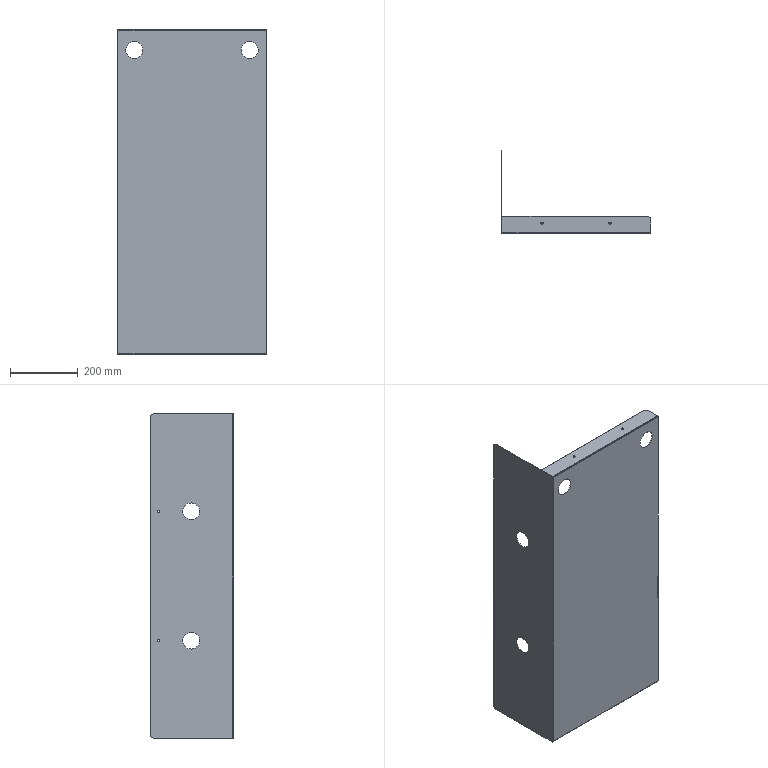Part | SolidWorks | features BaseBody 1 | 1 solid | 48 faces | box 440 x 245 x 955 mm | volume 1029152 mm3 | cylinder 30 | plane 18 | commonest cylinder face diameters 6.6 x12 50 x8 20 x4 1 x3 4 x3
STEP:
#1=CARTESIAN_POINT('',(50.,0.,870.));
#2=VERTEX_POINT('',#1);
#3=CARTESIAN_POINT('',(50.,0.,920.));
#4=VERTEX_POINT('',#3);
#5=CARTESIAN_POINT('',(50.,0.,895.));
#6=DIRECTION('',(0.,1.,0.));
#7=DIRECTION('',(0.,0.,1.));
#8=AXIS2_PLACEMENT_3D('',#5,#6,#7);
#9=CIRCLE('',#8,25.);
#10=EDGE_CURVE('',#2,#4,#9,.T.);
#11=ORIENTED_EDGE('',*,*,#10,.F.);
#12=CARTESIAN_POINT('',(50.,1.5,870.));
#13=VERTEX_POINT('',#12);
#14=CARTESIAN_POINT('',(50.,1.5,870.));
#15=DIRECTION('',(0.,1.,0.));
#16=VECTOR('',#15,1000.);
#17=LINE('',#14,#16);
#18=EDGE_CURVE('',#2,#13,#17,.T.);
#19=ORIENTED_EDGE('',*,*,#18,.T.);
#20=CARTESIAN_POINT('',(50.,1.5,920.));
#21=VERTEX_POINT('',#20);
#22=CARTESIAN_POINT('',(50.,1.5,895.));
#23=DIRECTION('',(0.,-1.,0.));
#24=DIRECTION('',(0.,0.,1.));
#25=AXIS2_PLACEMENT_3D('',#22,#23,#24);
#26=CIRCLE('',#25,25.);
#27=EDGE_CURVE('',#21,#13,#26,.T.);
#28=ORIENTED_EDGE('',*,*,#27,.F.);
#29=CARTESIAN_POINT('',(50.,1.5,920.));
#30=DIRECTION('',(0.,1.,0.));
#31=VECTOR('',#30,1000.);
#32=LINE('',#29,#31);
#33=EDGE_CURVE('',#4,#21,#32,.T.);
#34=ORIENTED_EDGE('',*,*,#33,.F.);
#35=EDGE_LOOP('',(#11,#19,#28,#34));
#36=FACE_OUTER_BOUND('',#35,.T.);
#37=CARTESIAN_POINT('',(50.,1.5,895.));
#38=DIRECTION('',(0.,1.,0.));
#39=DIRECTION('',(0.,0.,1.));
#40=AXIS2_PLACEMENT_3D('',#37,#38,#39);
#41=CYLINDRICAL_SURFACE('',#40,25.);
#42=ADVANCED_FACE('',(#36),#41,.F.);
#43=CARTESIAN_POINT('',(390.,0.,870.));
#44=VERTEX_POINT('',#43);
#45=CARTESIAN_POINT('',(390.,0.,920.));
#46=VERTEX_POINT('',#45);
#47=CARTESIAN_POINT('',(390.,0.,895.));
#48=DIRECTION('',(0.,1.,0.));
#49=DIRECTION('',(0.,0.,1.));
#50=AXIS2_PLACEMENT_3D('',#47,#48,#49);
#51=CIRCLE('',#50,25.);
#52=EDGE_CURVE('',#44,#46,#51,.T.);
#53=ORIENTED_EDGE('',*,*,#52,.F.);
#54=CARTESIAN_POINT('',(390.,1.5,870.));
#55=VERTEX_POINT('',#54);
#56=CARTESIAN_POINT('',(390.,1.5,870.));
#57=DIRECTION('',(0.,1.,0.));
#58=VECTOR('',#57,1000.);
#59=LINE('',#56,#58);
#60=EDGE_CURVE('',#44,#55,#59,.T.);
#61=ORIENTED_EDGE('',*,*,#60,.T.);
#62=CARTESIAN_POINT('',(390.,1.5,920.));
#63=VERTEX_POINT('',#62);
#64=CARTESIAN_POINT('',(390.,1.5,895.));
#65=DIRECTION('',(0.,-1.,0.));
#66=DIRECTION('',(0.,0.,1.));
#67=AXIS2_PLACEMENT_3D('',#64,#65,#66);
#68=CIRCLE('',#67,25.);
#69=EDGE_CURVE('',#63,#55,#68,.T.);
#70=ORIENTED_EDGE('',*,*,#69,.F.);
#71=CARTESIAN_POINT('',(390.,1.5,920.));
#72=DIRECTION('',(0.,1.,0.));
#73=VECTOR('',#72,1000.);
#74=LINE('',#71,#73);
#75=EDGE_CURVE('',#46,#63,#74,.T.);
#76=ORIENTED_EDGE('',*,*,#75,.F.);
#77=EDGE_LOOP('',(#53,#61,#70,#76));
#78=FACE_OUTER_BOUND('',#77,.T.);
#79=CARTESIAN_POINT('',(390.,1.5,895.));
#80=DIRECTION('',(0.,1.,0.));
#81=DIRECTION('',(0.,0.,1.));
#82=AXIS2_PLACEMENT_3D('',#79,#80,#81);
#83=CYLINDRICAL_SURFACE('',#82,25.);
#84=ADVANCED_FACE('',(#78),#83,.F.);
#85=CARTESIAN_POINT('',(316.7,30.,953.5));
#86=VERTEX_POINT('',#85);
#87=CARTESIAN_POINT('',(323.3,30.,953.5));
#88=VERTEX_POINT('',#87);
#89=CARTESIAN_POINT('',(320.,30.,953.5));
#90=DIRECTION('',(0.,0.,1.));
#91=DIRECTION('',(1.,0.,0.));
#92=AXIS2_PLACEMENT_3D('',#89,#90,#91);
#93=CIRCLE('',#92,3.3);
#94=EDGE_CURVE('',#86,#88,#93,.T.);
#95=ORIENTED_EDGE('',*,*,#94,.F.);
#96=CARTESIAN_POINT('',(316.7,30.,955.));
#97=VERTEX_POINT('',#96);
#98=CARTESIAN_POINT('',(316.7,30.,955.));
#99=DIRECTION('',(0.,0.,1.));
#100=VECTOR('',#99,1000.);
#101=LINE('',#98,#100);
#102=EDGE_CURVE('',#86,#97,#101,.T.);
#103=ORIENTED_EDGE('',*,*,#102,.T.);
#104=CARTESIAN_POINT('',(323.3,30.,955.));
#105=VERTEX_POINT('',#104);
#106=CARTESIAN_POINT('',(320.,30.,955.));
#107=DIRECTION('',(0.,0.,-1.));
#108=DIRECTION('',(1.,0.,0.));
#109=AXIS2_PLACEMENT_3D('',#106,#107,#108);
#110=CIRCLE('',#109,3.3);
#111=EDGE_CURVE('',#105,#97,#110,.T.);
#112=ORIENTED_EDGE('',*,*,#111,.F.);
#113=CARTESIAN_POINT('',(323.3,30.,955.));
#114=DIRECTION('',(0.,0.,1.));
#115=VECTOR('',#114,1000.);
#116=LINE('',#113,#115);
#117=EDGE_CURVE('',#88,#105,#116,.T.);
#118=ORIENTED_EDGE('',*,*,#117,.F.);
#119=EDGE_LOOP('',(#95,#103,#112,#118));
#120=FACE_OUTER_BOUND('',#119,.T.);
#121=CARTESIAN_POINT('',(320.,30.,955.));
#122=DIRECTION('',(0.,0.,1.));
#123=DIRECTION('',(1.,0.,0.));
#124=AXIS2_PLACEMENT_3D('',#121,#122,#123);
#125=CYLINDRICAL_SURFACE('',#124,3.3);
#126=ADVANCED_FACE('',(#120),#125,.F.);
#127=CARTESIAN_POINT('',(116.7,30.,953.5));
#128=VERTEX_POINT('',#127);
#129=CARTESIAN_POINT('',(123.3,30.,953.5));
#130=VERTEX_POINT('',#129);
#131=CARTESIAN_POINT('',(120.,30.,953.5));
#132=DIRECTION('',(0.,0.,1.));
#133=DIRECTION('',(1.,0.,0.));
#134=AXIS2_PLACEMENT_3D('',#131,#132,#133);
#135=CIRCLE('',#134,3.3);
#136=EDGE_CURVE('',#128,#130,#135,.T.);
#137=ORIENTED_EDGE('',*,*,#136,.F.);
#138=CARTESIAN_POINT('',(116.7,30.,955.));
#139=VERTEX_POINT('',#138);
#140=CARTESIAN_POINT('',(116.7,30.,955.));
#141=DIRECTION('',(0.,0.,1.));
#142=VECTOR('',#141,1000.);
#143=LINE('',#140,#142);
#144=EDGE_CURVE('',#128,#139,#143,.T.);
#145=ORIENTED_EDGE('',*,*,#144,.T.);
#146=CARTESIAN_POINT('',(123.3,30.,955.));
#147=VERTEX_POINT('',#146);
#148=CARTESIAN_POINT('',(120.,30.,955.));
#149=DIRECTION('',(0.,0.,-1.));
#150=DIRECTION('',(1.,0.,0.));
#151=AXIS2_PLACEMENT_3D('',#148,#149,#150);
#152=CIRCLE('',#151,3.3);
#153=EDGE_CURVE('',#147,#139,#152,.T.);
#154=ORIENTED_EDGE('',*,*,#153,.F.);
#155=CARTESIAN_POINT('',(123.3,30.,955.));
#156=DIRECTION('',(0.,0.,1.));
#157=VECTOR('',#156,1000.);
#158=LINE('',#155,#157);
#159=EDGE_CURVE('',#130,#147,#158,.T.);
#160=ORIENTED_EDGE('',*,*,#159,.F.);
#161=EDGE_LOOP('',(#137,#145,#154,#160));
#162=FACE_OUTER_BOUND('',#161,.T.);
#163=CARTESIAN_POINT('',(120.,30.,955.));
#164=DIRECTION('',(0.,0.,1.));
#165=DIRECTION('',(1.,0.,0.));
#166=AXIS2_PLACEMENT_3D('',#163,#164,#165);
#167=CYLINDRICAL_SURFACE('',#166,3.3);
#168=ADVANCED_FACE('',(#162),#167,.F.);
#169=CARTESIAN_POINT('',(0.,125.,312.5));
#170=VERTEX_POINT('',#169);
#171=CARTESIAN_POINT('',(0.,125.,262.5));
#172=VERTEX_POINT('',#171);
#173=CARTESIAN_POINT('',(0.,125.,287.5));
#174=DIRECTION('',(1.,0.,0.));
#175=DIRECTION('',(0.,0.,-1.));
#176=AXIS2_PLACEMENT_3D('',#173,#174,#175);
#177=CIRCLE('',#176,25.);
#178=EDGE_CURVE('',#170,#172,#177,.T.);
#179=ORIENTED_EDGE('',*,*,#178,.F.);
#180=CARTESIAN_POINT('',(1.5,125.,312.5));
#181=VERTEX_POINT('',#180);
#182=CARTESIAN_POINT('',(1.5,125.,312.5));
#183=DIRECTION('',(1.,0.,0.));
#184=VECTOR('',#183,1000.);
#185=LINE('',#182,#184);
#186=EDGE_CURVE('',#170,#181,#185,.T.);
#187=ORIENTED_EDGE('',*,*,#186,.T.);
#188=CARTESIAN_POINT('',(1.5,125.,262.5));
#189=VERTEX_POINT('',#188);
#190=CARTESIAN_POINT('',(1.5,125.,287.5));
#191=DIRECTION('',(-1.,0.,0.));
#192=DIRECTION('',(0.,0.,-1.));
#193=AXIS2_PLACEMENT_3D('',#190,#191,#192);
#194=CIRCLE('',#193,25.);
#195=EDGE_CURVE('',#189,#181,#194,.T.);
#196=ORIENTED_EDGE('',*,*,#195,.F.);
#197=CARTESIAN_POINT('',(1.5,125.,262.5));
#198=DIRECTION('',(1.,0.,0.));
#199=VECTOR('',#198,1000.);
#200=LINE('',#197,#199);
#201=EDGE_CURVE('',#172,#189,#200,.T.);
#202=ORIENTED_EDGE('',*,*,#201,.F.);
#203=EDGE_LOOP('',(#179,#187,#196,#202));
#204=FACE_OUTER_BOUND('',#203,.T.);
#205=CARTESIAN_POINT('',(1.5,125.,287.5));
#206=DIRECTION('',(1.,0.,0.));
#207=DIRECTION('',(0.,0.,-1.));
#208=AXIS2_PLACEMENT_3D('',#205,#206,#207);
#209=CYLINDRICAL_SURFACE('',#208,25.);
#210=ADVANCED_FACE('',(#204),#209,.F.);
#211=CARTESIAN_POINT('',(0.,125.,692.5));
#212=VERTEX_POINT('',#211);
#213=CARTESIAN_POINT('',(0.,125.,642.5));
#214=VERTEX_POINT('',#213);
#215=CARTESIAN_POINT('',(0.,125.,667.5));
#216=DIRECTION('',(1.,0.,0.));
#217=DIRECTION('',(0.,0.,-1.));
#218=AXIS2_PLACEMENT_3D('',#215,#216,#217);
#219=CIRCLE('',#218,25.);
#220=EDGE_CURVE('',#212,#214,#219,.T.);
#221=ORIENTED_EDGE('',*,*,#220,.F.);
#222=CARTESIAN_POINT('',(1.5,125.,692.5));
#223=VERTEX_POINT('',#222);
#224=CARTESIAN_POINT('',(1.5,125.,692.5));
#225=DIRECTION('',(1.,0.,0.));
#226=VECTOR('',#225,1000.);
#227=LINE('',#224,#226);
#228=EDGE_CURVE('',#212,#223,#227,.T.);
#229=ORIENTED_EDGE('',*,*,#228,.T.);
#230=CARTESIAN_POINT('',(1.5,125.,642.5));
#231=VERTEX_POINT('',#230);
#232=CARTESIAN_POINT('',(1.5,125.,667.5));
#233=DIRECTION('',(-1.,0.,0.));
#234=DIRECTION('',(0.,0.,-1.));
#235=AXIS2_PLACEMENT_3D('',#232,#233,#234);
#236=CIRCLE('',#235,25.);
#237=EDGE_CURVE('',#231,#223,#236,.T.);
#238=ORIENTED_EDGE('',*,*,#237,.F.);
#239=CARTESIAN_POINT('',(1.5,125.,642.5));
#240=DIRECTION('',(1.,0.,0.));
#241=VECTOR('',#240,1000.);
#242=LINE('',#239,#241);
#243=EDGE_CURVE('',#214,#231,#242,.T.);
#244=ORIENTED_EDGE('',*,*,#243,.F.);
#245=EDGE_LOOP('',(#221,#229,#238,#244));
#246=FACE_OUTER_BOUND('',#245,.T.);
#247=CARTESIAN_POINT('',(1.5,125.,667.5));
#248=DIRECTION('',(1.,0.,0.));
#249=DIRECTION('',(0.,0.,-1.));
#250=AXIS2_PLACEMENT_3D('',#247,#248,#249);
#251=CYLINDRICAL_SURFACE('',#250,25.);
#252=ADVANCED_FACE('',(#246),#251,.F.);
#253=CARTESIAN_POINT('',(0.,220.,290.8));
#254=VERTEX_POINT('',#253);
#255=CARTESIAN_POINT('',(0.,220.,284.2));
#256=VERTEX_POINT('',#255);
#257=CARTESIAN_POINT('',(0.,220.,287.5));
#258=DIRECTION('',(1.,0.,0.));
#259=DIRECTION('',(0.,0.,-1.));
#260=AXIS2_PLACEMENT_3D('',#257,#258,#259);
#261=CIRCLE('',#260,3.3);
#262=EDGE_CURVE('',#254,#256,#261,.T.);
#263=ORIENTED_EDGE('',*,*,#262,.F.);
#264=CARTESIAN_POINT('',(1.5,220.,290.8));
#265=VERTEX_POINT('',#264);
#266=CARTESIAN_POINT('',(1.5,220.,290.8));
#267=DIRECTION('',(1.,0.,0.));
#268=VECTOR('',#267,1000.);
#269=LINE('',#266,#268);
#270=EDGE_CURVE('',#254,#265,#269,.T.);
#271=ORIENTED_EDGE('',*,*,#270,.T.);
#272=CARTESIAN_POINT('',(1.5,220.,284.2));
#273=VERTEX_POINT('',#272);
#274=CARTESIAN_POINT('',(1.5,220.,287.5));
#275=DIRECTION('',(-1.,0.,0.));
#276=DIRECTION('',(0.,0.,-1.));
#277=AXIS2_PLACEMENT_3D('',#274,#275,#276);
#278=CIRCLE('',#277,3.3);
#279=EDGE_CURVE('',#273,#265,#278,.T.);
#280=ORIENTED_EDGE('',*,*,#279,.F.);
#281=CARTESIAN_POINT('',(1.5,220.,284.2));
#282=DIRECTION('',(1.,0.,0.));
#283=VECTOR('',#282,1000.);
#284=LINE('',#281,#283);
#285=EDGE_CURVE('',#256,#273,#284,.T.);
#286=ORIENTED_EDGE('',*,*,#285,.F.);
#287=EDGE_LOOP('',(#263,#271,#280,#286));
#288=FACE_OUTER_BOUND('',#287,.T.);
#289=CARTESIAN_POINT('',(1.5,220.,287.5));
#290=DIRECTION('',(1.,0.,0.));
#291=DIRECTION('',(0.,0.,-1.));
#292=AXIS2_PLACEMENT_3D('',#289,#290,#291);
#293=CYLINDRICAL_SURFACE('',#292,3.3);
#294=ADVANCED_FACE('',(#288),#293,.F.);
#295=CARTESIAN_POINT('',(0.,220.,670.8));
#296=VERTEX_POINT('',#295);
#297=CARTESIAN_POINT('',(0.,220.,664.2));
#298=VERTEX_POINT('',#297);
#299=CARTESIAN_POINT('',(0.,220.,667.5));
#300=DIRECTION('',(1.,0.,0.));
#301=DIRECTION('',(0.,0.,-1.));
#302=AXIS2_PLACEMENT_3D('',#299,#300,#301);
#303=CIRCLE('',#302,3.3);
#304=EDGE_CURVE('',#296,#298,#303,.T.);
#305=ORIENTED_EDGE('',*,*,#304,.F.);
#306=CARTESIAN_POINT('',(1.5,220.,670.8));
#307=VERTEX_POINT('',#306);
#308=CARTESIAN_POINT('',(1.5,220.,670.8));
#309=DIRECTION('',(1.,0.,0.));
#310=VECTOR('',#309,1000.);
#311=LINE('',#308,#310);
#312=EDGE_CURVE('',#296,#307,#311,.T.);
#313=ORIENTED_EDGE('',*,*,#312,.T.);
#314=CARTESIAN_POINT('',(1.5,220.,664.2));
#315=VERTEX_POINT('',#314);
#316=CARTESIAN_POINT('',(1.5,220.,667.5));
#317=DIRECTION('',(-1.,0.,0.));
#318=DIRECTION('',(0.,0.,-1.));
#319=AXIS2_PLACEMENT_3D('',#316,#317,#318);
#320=CIRCLE('',#319,3.3);
#321=EDGE_CURVE('',#315,#307,#320,.T.);
#322=ORIENTED_EDGE('',*,*,#321,.F.);
#323=CARTESIAN_POINT('',(1.5,220.,664.2));
#324=DIRECTION('',(1.,0.,0.));
#325=VECTOR('',#324,1000.);
#326=LINE('',#323,#325);
#327=EDGE_CURVE('',#298,#315,#326,.T.);
#328=ORIENTED_EDGE('',*,*,#327,.F.);
#329=EDGE_LOOP('',(#305,#313,#322,#328));
#330=FACE_OUTER_BOUND('',#329,.T.);
#331=CARTESIAN_POINT('',(1.5,220.,667.5));
#332=DIRECTION('',(1.,0.,0.));
#333=DIRECTION('',(0.,0.,-1.));
#334=AXIS2_PLACEMENT_3D('',#331,#332,#333);
#335=CYLINDRICAL_SURFACE('',#334,3.3);
#336=ADVANCED_FACE('',(#330),#335,.F.);
#337=CARTESIAN_POINT('',(316.7,30.,0.));
#338=VERTEX_POINT('',#337);
#339=CARTESIAN_POINT('',(323.3,30.,0.));
#340=VERTEX_POINT('',#339);
#341=CARTESIAN_POINT('',(320.,30.,0.));
#342=DIRECTION('',(0.,0.,1.));
#343=DIRECTION('',(1.,0.,0.));
#344=AXIS2_PLACEMENT_3D('',#341,#342,#343);
#345=CIRCLE('',#344,3.3);
#346=EDGE_CURVE('',#338,#340,#345,.T.);
#347=ORIENTED_EDGE('',*,*,#346,.F.);
#348=CARTESIAN_POINT('',(316.7,30.,1.5));
#349=VERTEX_POINT('',#348);
#350=CARTESIAN_POINT('',(316.7,30.,955.));
#351=DIRECTION('',(0.,0.,1.));
#352=VECTOR('',#351,1000.);
#353=LINE('',#350,#352);
#354=EDGE_CURVE('',#338,#349,#353,.T.);
#355=ORIENTED_EDGE('',*,*,#354,.T.);
#356=CARTESIAN_POINT('',(323.3,30.,1.5));
#357=VERTEX_POINT('',#356);
#358=CARTESIAN_POINT('',(320.,30.,1.5));
#359=DIRECTION('',(0.,0.,-1.));
#360=DIRECTION('',(1.,0.,0.));
#361=AXIS2_PLACEMENT_3D('',#358,#359,#360);
#362=CIRCLE('',#361,3.3);
#363=EDGE_CURVE('',#357,#349,#362,.T.);
#364=ORIENTED_EDGE('',*,*,#363,.F.);
#365=CARTESIAN_POINT('',(323.3,30.,955.));
#366=DIRECTION('',(0.,0.,1.));
#367=VECTOR('',#366,1000.);
#368=LINE('',#365,#367);
#369=EDGE_CURVE('',#340,#357,#368,.T.);
#370=ORIENTED_EDGE('',*,*,#369,.F.);
#371=EDGE_LOOP('',(#347,#355,#364,#370));
#372=FACE_OUTER_BOUND('',#371,.T.);
#373=CARTESIAN_POINT('',(320.,30.,955.));
#374=DIRECTION('',(0.,0.,1.));
#375=DIRECTION('',(1.,0.,0.));
#376=AXIS2_PLACEMENT_3D('',#373,#374,#375);
#377=CYLINDRICAL_SURFACE('',#376,3.3);
#378=ADVANCED_FACE('',(#372),#377,.F.);
#379=CARTESIAN_POINT('',(116.7,30.,0.));
#380=VERTEX_POINT('',#379);
#381=CARTESIAN_POINT('',(123.3,30.,0.));
#382=VERTEX_POINT('',#381);
#383=CARTESIAN_POINT('',(120.,30.,0.));
#384=DIRECTION('',(0.,0.,1.));
#385=DIRECTION('',(1.,0.,0.));
#386=AXIS2_PLACEMENT_3D('',#383,#384,#385);
#387=CIRCLE('',#386,3.3);
#388=EDGE_CURVE('',#380,#382,#387,.T.);
#389=ORIENTED_EDGE('',*,*,#388,.F.);
#390=CARTESIAN_POINT('',(116.7,30.,1.5));
#391=VERTEX_POINT('',#390);
#392=CARTESIAN_POINT('',(116.7,30.,955.));
#393=DIRECTION('',(0.,0.,1.));
#394=VECTOR('',#393,1000.);
#395=LINE('',#392,#394);
#396=EDGE_CURVE('',#380,#391,#395,.T.);
#397=ORIENTED_EDGE('',*,*,#396,.T.);
#398=CARTESIAN_POINT('',(123.3,30.,1.5));
#399=VERTEX_POINT('',#398);
#400=CARTESIAN_POINT('',(120.,30.,1.5));
#401=DIRECTION('',(0.,0.,-1.));
#402=DIRECTION('',(1.,0.,0.));
#403=AXIS2_PLACEMENT_3D('',#400,#401,#402);
#404=CIRCLE('',#403,3.3);
#405=EDGE_CURVE('',#399,#391,#404,.T.);
#406=ORIENTED_EDGE('',*,*,#405,.F.);
#407=CARTESIAN_POINT('',(123.3,30.,955.));
#408=DIRECTION('',(0.,0.,1.));
#409=VECTOR('',#408,1000.);
#410=LINE('',#407,#409);
#411=EDGE_CURVE('',#382,#399,#410,.T.);
#412=ORIENTED_EDGE('',*,*,#411,.F.);
#413=EDGE_LOOP('',(#389,#397,#406,#412));
#414=FACE_OUTER_BOUND('',#413,.T.);
#415=CARTESIAN_POINT('',(120.,30.,955.));
#416=DIRECTION('',(0.,0.,1.));
#417=DIRECTION('',(1.,0.,0.));
#418=AXIS2_PLACEMENT_3D('',#415,#416,#417);
#419=CYLINDRICAL_SURFACE('',#418,3.3);
#420=ADVANCED_FACE('',(#414),#419,.F.);
#421=CARTESIAN_POINT('',(2.,1.5,2.));
#422=VERTEX_POINT('',#421);
#423=CARTESIAN_POINT('',(2.,1.5,953.));
#424=VERTEX_POINT('',#423);
#425=CARTESIAN_POINT('',(2.,1.5,955.));
#426=DIRECTION('',(0.,0.,1.));
#427=VECTOR('',#426,1000.);
#428=LINE('',#425,#427);
#429=EDGE_CURVE('',#422,#424,#428,.T.);
#430=ORIENTED_EDGE('',*,*,#429,.T.);
#431=CARTESIAN_POINT('',(440.,1.5,953.));
#432=VERTEX_POINT('',#431);
#433=CARTESIAN_POINT('',(0.,1.5,953.));
#434=DIRECTION('',(1.,0.,0.));
#435=VECTOR('',#434,1000.);
#436=LINE('',#433,#435);
#437=EDGE_CURVE('',#424,#432,#436,.T.);
#438=ORIENTED_EDGE('',*,*,#437,.T.);
#439=CARTESIAN_POINT('',(440.,1.5,2.));
#440=VERTEX_POINT('',#439);
#441=CARTESIAN_POINT('',(440.,1.5,955.));
#442=DIRECTION('',(0.,0.,-1.));
#443=VECTOR('',#442,1000.);
#444=LINE('',#441,#443);
#445=EDGE_CURVE('',#432,#440,#444,.T.);
#446=ORIENTED_EDGE('',*,*,#445,.T.);
#447=CARTESIAN_POINT('',(0.,1.5,2.));
#448=DIRECTION('',(-1.,0.,0.));
#449=VECTOR('',#448,1000.);
#450=LINE('',#447,#449);
#451=EDGE_CURVE('',#440,#422,#450,.T.);
#452=ORIENTED_EDGE('',*,*,#451,.T.);
#453=EDGE_LOOP('',(#430,#438,#446,#452));
#454=FACE_OUTER_BOUND('',#453,.T.);
#455=ORIENTED_EDGE('',*,*,#27,.T.);
#456=CARTESIAN_POINT('',(50.,1.5,895.));
#457=DIRECTION('',(0.,-1.,0.));
#458=DIRECTION('',(0.,0.,1.));
#459=AXIS2_PLACEMENT_3D('',#456,#457,#458);
#460=CIRCLE('',#459,25.);
#461=EDGE_CURVE('',#13,#21,#460,.T.);
#462=ORIENTED_EDGE('',*,*,#461,.T.);
#463=EDGE_LOOP('',(#455,#462));
#464=FACE_BOUND('',#463,.T.);
#465=ORIENTED_EDGE('',*,*,#69,.T.);
#466=CARTESIAN_POINT('',(390.,1.5,895.));
#467=DIRECTION('',(0.,-1.,0.));
#468=DIRECTION('',(0.,0.,1.));
#469=AXIS2_PLACEMENT_3D('',#466,#467,#468);
#470=CIRCLE('',#469,25.);
#471=EDGE_CURVE('',#55,#63,#470,.T.);
#472=ORIENTED_EDGE('',*,*,#471,.T.);
#473=EDGE_LOOP('',(#465,#472));
#474=FACE_BOUND('',#473,.T.);
#475=CARTESIAN_POINT('',(0.,1.5,955.));
#476=DIRECTION('',(0.,1.,0.));
#477=DIRECTION('',(0.,0.,1.));
#478=AXIS2_PLACEMENT_3D('',#475,#476,#477);
#479=PLANE('',#478);
#480=ADVANCED_FACE('',(#454,#464,#474),#479,.T.);
#481=CARTESIAN_POINT('',(2.,2.,953.5));
#482=VERTEX_POINT('',#481);
#483=CARTESIAN_POINT('',(2.,2.,953.));
#484=DIRECTION('',(1.,0.,0.));
#485=DIRECTION('',(0.,0.,-1.));
#486=AXIS2_PLACEMENT_3D('',#483,#484,#485);
#487=CIRCLE('',#486,0.5);
#488=EDGE_CURVE('',#482,#424,#487,.T.);
#489=ORIENTED_EDGE('',*,*,#488,.F.);
#490=CARTESIAN_POINT('',(440.,2.,953.5));
#491=VERTEX_POINT('',#490);
#492=CARTESIAN_POINT('',(440.,2.,953.5));
#493=DIRECTION('',(-1.,0.,0.));
#494=VECTOR('',#493,1000.);
#495=LINE('',#492,#494);
#496=EDGE_CURVE('',#491,#482,#495,.T.);
#497=ORIENTED_EDGE('',*,*,#496,.F.);
#498=CARTESIAN_POINT('',(440.,2.,953.));
#499=DIRECTION('',(1.,0.,0.));
#500=DIRECTION('',(0.,0.,-1.));
#501=AXIS2_PLACEMENT_3D('',#498,#499,#500);
#502=CIRCLE('',#501,0.5);
#503=EDGE_CURVE('',#491,#432,#502,.T.);
#504=ORIENTED_EDGE('',*,*,#503,.T.);
#505=ORIENTED_EDGE('',*,*,#437,.F.);
#506=EDGE_LOOP('',(#489,#497,#504,#505));
#507=FACE_OUTER_BOUND('',#506,.T.);
#508=CARTESIAN_POINT('',(440.,2.,953.));
#509=DIRECTION('',(1.,0.,0.));
#510=DIRECTION('',(0.,0.,-1.));
#511=AXIS2_PLACEMENT_3D('',#508,#509,#510);
#512=CYLINDRICAL_SURFACE('',#511,0.5);
#513=ADVANCED_FACE('',(#507),#512,.F.);
#514=CARTESIAN_POINT('',(1.5,2.,955.));
#515=VERTEX_POINT('',#514);
#516=CARTESIAN_POINT('',(1.5,2.,0.));
#517=VERTEX_POINT('',#516);
#518=CARTESIAN_POINT('',(1.5,2.,955.));
#519=DIRECTION('',(0.,0.,-1.));
#520=VECTOR('',#519,1000.);
#521=LINE('',#518,#520);
#522=EDGE_CURVE('',#515,#517,#521,.T.);
#523=ORIENTED_EDGE('',*,*,#522,.F.);
#524=CARTESIAN_POINT('',(2.,1.5,955.));
#525=VERTEX_POINT('',#524);
#526=CARTESIAN_POINT('',(2.,2.,955.));
#527=DIRECTION('',(0.,0.,-1.));
#528=DIRECTION('',(-1.,0.,0.));
#529=AXIS2_PLACEMENT_3D('',#526,#527,#528);
#530=CIRCLE('',#529,0.5);
#531=EDGE_CURVE('',#525,#515,#530,.T.);
#532=ORIENTED_EDGE('',*,*,#531,.F.);
#533=CARTESIAN_POINT('',(2.,1.5,954.936));
#534=VERTEX_POINT('',#533);
#535=CARTESIAN_POINT('',(2.,1.5,953.));
#536=DIRECTION('',(0.,0.,1.));
#537=VECTOR('',#536,1000.);
#538=LINE('',#535,#537);
#539=EDGE_CURVE('',#534,#525,#538,.T.);
#540=ORIENTED_EDGE('',*,*,#539,.F.);
#541=CARTESIAN_POINT('',(2.,1.5,955.));
#542=DIRECTION('',(0.,0.,1.));
#543=VECTOR('',#542,1000.);
#544=LINE('',#541,#543);
#545=EDGE_CURVE('',#424,#534,#544,.T.);
#546=ORIENTED_EDGE('',*,*,#545,.F.);
#547=ORIENTED_EDGE('',*,*,#429,.F.);
#548=CARTESIAN_POINT('',(2.,1.5,0.06351));
#549=VERTEX_POINT('',#548);
#550=CARTESIAN_POINT('',(2.,1.5,955.));
#551=DIRECTION('',(0.,0.,1.));
#552=VECTOR('',#551,1000.);
#553=LINE('',#550,#552);
#554=EDGE_CURVE('',#549,#422,#553,.T.);
#555=ORIENTED_EDGE('',*,*,#554,.F.);
#556=CARTESIAN_POINT('',(2.,1.5,0.));
#557=VERTEX_POINT('',#556);
#558=CARTESIAN_POINT('',(2.,1.5,0.));
#559=DIRECTION('',(0.,0.,1.));
#560=VECTOR('',#559,1000.);
#561=LINE('',#558,#560);
#562=EDGE_CURVE('',#557,#549,#561,.T.);
#563=ORIENTED_EDGE('',*,*,#562,.F.);
#564=CARTESIAN_POINT('',(2.,2.,0.));
#565=DIRECTION('',(0.,0.,1.));
#566=DIRECTION('',(-1.,0.,0.));
#567=AXIS2_PLACEMENT_3D('',#564,#565,#566);
#568=CIRCLE('',#567,0.5);
#569=EDGE_CURVE('',#517,#557,#568,.T.);
#570=ORIENTED_EDGE('',*,*,#569,.F.);
#571=EDGE_LOOP('',(#523,#532,#540,#546,#547,#555,#563,#570));
#572=FACE_OUTER_BOUND('',#571,.T.);
#573=CARTESIAN_POINT('',(2.,2.,955.));
#574=DIRECTION('',(0.,0.,-1.));
#575=DIRECTION('',(-1.,0.,0.));
#576=AXIS2_PLACEMENT_3D('',#573,#574,#575);
#577=CYLINDRICAL_SURFACE('',#576,0.5);
#578=ADVANCED_FACE('',(#572),#577,.F.);
#579=CARTESIAN_POINT('',(440.,2.,1.5));
#580=VERTEX_POINT('',#579);
#581=CARTESIAN_POINT('',(440.,2.,2.));
#582=DIRECTION('',(-1.,0.,0.));
#583=DIRECTION('',(0.,0.,1.));
#584=AXIS2_PLACEMENT_3D('',#581,#582,#583);
#585=CIRCLE('',#584,0.5);
#586=EDGE_CURVE('',#580,#440,#585,.T.);
#587=ORIENTED_EDGE('',*,*,#586,.F.);
#588=CARTESIAN_POINT('',(2.,2.,1.5));
#589=VERTEX_POINT('',#588);
#590=CARTESIAN_POINT('',(2.,2.,1.5));
#591=DIRECTION('',(1.,0.,0.));
#592=VECTOR('',#591,1000.);
#593=LINE('',#590,#592);
#594=EDGE_CURVE('',#589,#580,#593,.T.);
#595=ORIENTED_EDGE('',*,*,#594,.F.);
#596=CARTESIAN_POINT('',(2.,2.,2.));
#597=DIRECTION('',(1.,0.,0.));
#598=DIRECTION('',(0.,0.,1.));
#599=AXIS2_PLACEMENT_3D('',#596,#597,#598);
#600=CIRCLE('',#599,0.5);
#601=EDGE_CURVE('',#422,#589,#600,.T.);
#602=ORIENTED_EDGE('',*,*,#601,.F.);
#603=ORIENTED_EDGE('',*,*,#451,.F.);
#604=EDGE_LOOP('',(#587,#595,#602,#603));
#605=FACE_OUTER_BOUND('',#604,.T.);
#606=CARTESIAN_POINT('',(2.,2.,2.));
#607=DIRECTION('',(-1.,0.,0.));
#608=DIRECTION('',(0.,0.,1.));
#609=AXIS2_PLACEMENT_3D('',#606,#607,#608);
#610=CYLINDRICAL_SURFACE('',#609,0.5);
#611=ADVANCED_FACE('',(#605),#610,.F.);
#612=ORIENTED_EDGE('',*,*,#445,.F.);
#613=ORIENTED_EDGE('',*,*,#503,.F.);
#614=CARTESIAN_POINT('',(440.,40.,953.5));
#615=VERTEX_POINT('',#614);
#616=CARTESIAN_POINT('',(440.,0.,953.5));
#617=DIRECTION('',(0.,-1.,0.));
#618=VECTOR('',#617,1000.);
#619=LINE('',#616,#618);
#620=EDGE_CURVE('',#615,#491,#619,.T.);
#621=ORIENTED_EDGE('',*,*,#620,.F.);
#622=CARTESIAN_POINT('',(440.,40.,955.));
#623=VERTEX_POINT('',#622);
#624=CARTESIAN_POINT('',(440.,40.,955.));
#625=DIRECTION('',(0.,0.,-1.));
#626=VECTOR('',#625,1000.);
#627=LINE('',#624,#626);
#628=EDGE_CURVE('',#623,#615,#627,.T.);
#629=ORIENTED_EDGE('',*,*,#628,.F.);
#630=CARTESIAN_POINT('',(440.,2.,955.));
#631=VERTEX_POINT('',#630);
#632=CARTESIAN_POINT('',(440.,50.,955.));
#633=DIRECTION('',(0.,1.,0.));
#634=VECTOR('',#633,1000.);
#635=LINE('',#632,#634);
#636=EDGE_CURVE('',#631,#623,#635,.T.);
#637=ORIENTED_EDGE('',*,*,#636,.F.);
#638=CARTESIAN_POINT('',(440.,0.,953.));
#639=VERTEX_POINT('',#638);
#640=CARTESIAN_POINT('',(440.,2.,953.));
#641=DIRECTION('',(-1.,0.,0.));
#642=DIRECTION('',(0.,0.,-1.));
#643=AXIS2_PLACEMENT_3D('',#640,#641,#642);
#644=CIRCLE('',#643,2.);
#645=EDGE_CURVE('',#639,#631,#644,.T.);
#646=ORIENTED_EDGE('',*,*,#645,.F.);
#647=CARTESIAN_POINT('',(440.,0.,2.));
#648=VERTEX_POINT('',#647);
#649=CARTESIAN_POINT('',(440.,0.,955.));
#650=DIRECTION('',(0.,0.,-1.));
#651=VECTOR('',#650,1000.);
#652=LINE('',#649,#651);
#653=EDGE_CURVE('',#639,#648,#652,.T.);
#654=ORIENTED_EDGE('',*,*,#653,.T.);
#655=CARTESIAN_POINT('',(440.,2.,0.));
#656=VERTEX_POINT('',#655);
#657=CARTESIAN_POINT('',(440.,2.,2.));
#658=DIRECTION('',(-1.,0.,0.));
#659=DIRECTION('',(0.,0.,1.));
#660=AXIS2_PLACEMENT_3D('',#657,#658,#659);
#661=CIRCLE('',#660,2.);
#662=EDGE_CURVE('',#656,#648,#661,.T.);
#663=ORIENTED_EDGE('',*,*,#662,.F.);
#664=CARTESIAN_POINT('',(440.,40.,0.));
#665=VERTEX_POINT('',#664);
#666=CARTESIAN_POINT('',(440.,1.5,0.));
#667=DIRECTION('',(0.,-1.,0.));
#668=VECTOR('',#667,1000.);
#669=LINE('',#666,#668);
#670=EDGE_CURVE('',#665,#656,#669,.T.);
#671=ORIENTED_EDGE('',*,*,#670,.F.);
#672=CARTESIAN_POINT('',(440.,40.,1.5));
#673=VERTEX_POINT('',#672);
#674=CARTESIAN_POINT('',(440.,40.,0.));
#675=DIRECTION('',(0.,0.,-1.));
#676=VECTOR('',#675,1000.);
#677=LINE('',#674,#676);
#678=EDGE_CURVE('',#673,#665,#677,.T.);
#679=ORIENTED_EDGE('',*,*,#678,.F.);
#680=CARTESIAN_POINT('',(440.,0.,1.5));
#681=DIRECTION('',(0.,1.,0.));
#682=VECTOR('',#681,1000.);
#683=LINE('',#680,#682);
#684=EDGE_CURVE('',#580,#673,#683,.T.);
#685=ORIENTED_EDGE('',*,*,#684,.F.);
#686=ORIENTED_EDGE('',*,*,#586,.T.);
#687=EDGE_LOOP('',(#612,#613,#621,#629,#637,#646,#654,#663,#671,#679,#685,#686));
#688=FACE_OUTER_BOUND('',#687,.T.);
#689=CARTESIAN_POINT('',(440.,1.5,955.));
#690=DIRECTION('',(1.,0.,0.));
#691=DIRECTION('',(0.,0.,-1.));
#692=AXIS2_PLACEMENT_3D('',#689,#690,#691);
#693=PLANE('',#692);
#694=ADVANCED_FACE('',(#688),#693,.T.);
#695=ORIENTED_EDGE('',*,*,#18,.F.);
#696=CARTESIAN_POINT('',(50.,0.,895.));
#697=DIRECTION('',(0.,1.,0.));
#698=DIRECTION('',(0.,0.,1.));
#699=AXIS2_PLACEMENT_3D('',#696,#697,#698);
#700=CIRCLE('',#699,25.);
#701=EDGE_CURVE('',#4,#2,#700,.T.);
#702=ORIENTED_EDGE('',*,*,#701,.F.);
#703=ORIENTED_EDGE('',*,*,#33,.T.);
#704=ORIENTED_EDGE('',*,*,#461,.F.);
#705=EDGE_LOOP('',(#695,#702,#703,#704));
#706=FACE_OUTER_BOUND('',#705,.T.);
#707=CARTESIAN_POINT('',(50.,1.5,895.));
#708=DIRECTION('',(0.,1.,0.));
#709=DIRECTION('',(0.,0.,1.));
#710=AXIS2_PLACEMENT_3D('',#707,#708,#709);
#711=CYLINDRICAL_SURFACE('',#710,25.);
#712=ADVANCED_FACE('',(#706),#711,.F.);
#713=ORIENTED_EDGE('',*,*,#60,.F.);
#714=CARTESIAN_POINT('',(390.,0.,895.));
#715=DIRECTION('',(0.,1.,0.));
#716=DIRECTION('',(0.,0.,1.));
#717=AXIS2_PLACEMENT_3D('',#714,#715,#716);
#718=CIRCLE('',#717,25.);
#719=EDGE_CURVE('',#46,#44,#718,.T.);
#720=ORIENTED_EDGE('',*,*,#719,.F.);
#721=ORIENTED_EDGE('',*,*,#75,.T.);
#722=ORIENTED_EDGE('',*,*,#471,.F.);
#723=EDGE_LOOP('',(#713,#720,#721,#722));
#724=FACE_OUTER_BOUND('',#723,.T.);
#725=CARTESIAN_POINT('',(390.,1.5,895.));
#726=DIRECTION('',(0.,1.,0.));
#727=DIRECTION('',(0.,0.,1.));
#728=AXIS2_PLACEMENT_3D('',#725,#726,#727);
#729=CYLINDRICAL_SURFACE('',#728,25.);
#730=ADVANCED_FACE('',(#724),#729,.F.);
#731=ORIENTED_EDGE('',*,*,#496,.T.);
#732=CARTESIAN_POINT('',(2.,50.,953.5));
#733=VERTEX_POINT('',#732);
#734=CARTESIAN_POINT('',(2.,0.,953.5));
#735=DIRECTION('',(0.,1.,0.));
#736=VECTOR('',#735,1000.);
#737=LINE('',#734,#736);
#738=EDGE_CURVE('',#482,#733,#737,.T.);
#739=ORIENTED_EDGE('',*,*,#738,.T.);
#740=CARTESIAN_POINT('',(430.,50.,953.5));
#741=VERTEX_POINT('',#740);
#742=CARTESIAN_POINT('',(0.,50.,953.5));
#743=DIRECTION('',(1.,0.,0.));
#744=VECTOR('',#743,1000.);
#745=LINE('',#742,#744);
#746=EDGE_CURVE('',#733,#741,#745,.T.);
#747=ORIENTED_EDGE('',*,*,#746,.T.);
#748=CARTESIAN_POINT('',(430.,40.,953.5));
#749=DIRECTION('',(0.,0.,-1.));
#750=DIRECTION('',(-1.,0.,0.));
#751=AXIS2_PLACEMENT_3D('',#748,#749,#750);
#752=CIRCLE('',#751,10.);
#753=EDGE_CURVE('',#741,#615,#752,.T.);
#754=ORIENTED_EDGE('',*,*,#753,.T.);
#755=ORIENTED_EDGE('',*,*,#620,.T.);
#756=EDGE_LOOP('',(#731,#739,#747,#754,#755));
#757=FACE_OUTER_BOUND('',#756,.T.);
#758=CARTESIAN_POINT('',(320.,30.,953.5));
#759=DIRECTION('',(0.,0.,1.));
#760=DIRECTION('',(1.,0.,0.));
#761=AXIS2_PLACEMENT_3D('',#758,#759,#760);
#762=CIRCLE('',#761,3.3);
#763=EDGE_CURVE('',#88,#86,#762,.T.);
#764=ORIENTED_EDGE('',*,*,#763,.T.);
#765=ORIENTED_EDGE('',*,*,#94,.T.);
#766=EDGE_LOOP('',(#764,#765));
#767=FACE_BOUND('',#766,.T.);
#768=CARTESIAN_POINT('',(120.,30.,953.5));
#769=DIRECTION('',(0.,0.,1.));
#770=DIRECTION('',(1.,0.,0.));
#771=AXIS2_PLACEMENT_3D('',#768,#769,#770);
#772=CIRCLE('',#771,3.3);
#773=EDGE_CURVE('',#130,#128,#772,.T.);
#774=ORIENTED_EDGE('',*,*,#773,.T.);
#775=ORIENTED_EDGE('',*,*,#136,.T.);
#776=EDGE_LOOP('',(#774,#775));
#777=FACE_BOUND('',#776,.T.);
#778=CARTESIAN_POINT('',(0.,0.,953.5));
#779=DIRECTION('',(0.,0.,-1.));
#780=DIRECTION('',(-1.,0.,0.));
#781=AXIS2_PLACEMENT_3D('',#778,#779,#780);
#782=PLANE('',#781);
#783=ADVANCED_FACE('',(#757,#767,#777),#782,.T.);
#784=CARTESIAN_POINT('',(1.5,235.,955.));
#785=VERTEX_POINT('',#784);
#786=CARTESIAN_POINT('',(1.5,245.,955.));
#787=DIRECTION('',(0.,-1.,0.));
#788=VECTOR('',#787,1000.);
#789=LINE('',#786,#788);
#790=EDGE_CURVE('',#785,#515,#789,.T.);
#791=ORIENTED_EDGE('',*,*,#790,.T.);
#792=ORIENTED_EDGE('',*,*,#522,.T.);
#793=CARTESIAN_POINT('',(1.5,235.,0.));
#794=VERTEX_POINT('',#793);
#795=CARTESIAN_POINT('',(1.5,245.,0.));
#796=DIRECTION('',(0.,1.,0.));
#797=VECTOR('',#796,1000.);
#798=LINE('',#795,#797);
#799=EDGE_CURVE('',#517,#794,#798,.T.);
#800=ORIENTED_EDGE('',*,*,#799,.T.);
#801=CARTESIAN_POINT('',(1.5,245.,10.));
#802=VERTEX_POINT('',#801);
#803=CARTESIAN_POINT('',(1.5,235.,10.));
#804=DIRECTION('',(1.,0.,0.));
#805=DIRECTION('',(0.,0.,1.));
#806=AXIS2_PLACEMENT_3D('',#803,#804,#805);
#807=CIRCLE('',#806,10.);
#808=EDGE_CURVE('',#794,#802,#807,.T.);
#809=ORIENTED_EDGE('',*,*,#808,.T.);
#810=CARTESIAN_POINT('',(1.5,245.,945.));
#811=VERTEX_POINT('',#810);
#812=CARTESIAN_POINT('',(1.5,245.,955.));
#813=DIRECTION('',(0.,0.,1.));
#814=VECTOR('',#813,1000.);
#815=LINE('',#812,#814);
#816=EDGE_CURVE('',#802,#811,#815,.T.);
#817=ORIENTED_EDGE('',*,*,#816,.T.);
#818=CARTESIAN_POINT('',(1.5,235.,945.));
#819=DIRECTION('',(1.,0.,0.));
#820=DIRECTION('',(0.,0.,-1.));
#821=AXIS2_PLACEMENT_3D('',#818,#819,#820);
#822=CIRCLE('',#821,10.);
#823=EDGE_CURVE('',#811,#785,#822,.T.);
#824=ORIENTED_EDGE('',*,*,#823,.T.);
#825=EDGE_LOOP('',(#791,#792,#800,#809,#817,#824));
#826=FACE_OUTER_BOUND('',#825,.T.);
#827=ORIENTED_EDGE('',*,*,#195,.T.);
#828=CARTESIAN_POINT('',(1.5,125.,287.5));
#829=DIRECTION('',(-1.,0.,0.));
#830=DIRECTION('',(0.,0.,-1.));
#831=AXIS2_PLACEMENT_3D('',#828,#829,#830);
#832=CIRCLE('',#831,25.);
#833=EDGE_CURVE('',#181,#189,#832,.T.);
#834=ORIENTED_EDGE('',*,*,#833,.T.);
#835=EDGE_LOOP('',(#827,#834));
#836=FACE_BOUND('',#835,.T.);
#837=ORIENTED_EDGE('',*,*,#237,.T.);
#838=CARTESIAN_POINT('',(1.5,125.,667.5));
#839=DIRECTION('',(-1.,0.,0.));
#840=DIRECTION('',(0.,0.,-1.));
#841=AXIS2_PLACEMENT_3D('',#838,#839,#840);
#842=CIRCLE('',#841,25.);
#843=EDGE_CURVE('',#223,#231,#842,.T.);
#844=ORIENTED_EDGE('',*,*,#843,.T.);
#845=EDGE_LOOP('',(#837,#844));
#846=FACE_BOUND('',#845,.T.);
#847=ORIENTED_EDGE('',*,*,#279,.T.);
#848=CARTESIAN_POINT('',(1.5,220.,287.5));
#849=DIRECTION('',(-1.,0.,0.));
#850=DIRECTION('',(0.,0.,-1.));
#851=AXIS2_PLACEMENT_3D('',#848,#849,#850);
#852=CIRCLE('',#851,3.3);
#853=EDGE_CURVE('',#265,#273,#852,.T.);
#854=ORIENTED_EDGE('',*,*,#853,.T.);
#855=EDGE_LOOP('',(#847,#854));
#856=FACE_BOUND('',#855,.T.);
#857=ORIENTED_EDGE('',*,*,#321,.T.);
#858=CARTESIAN_POINT('',(1.5,220.,667.5));
#859=DIRECTION('',(-1.,0.,0.));
#860=DIRECTION('',(0.,0.,-1.));
#861=AXIS2_PLACEMENT_3D('',#858,#859,#860);
#862=CIRCLE('',#861,3.3);
#863=EDGE_CURVE('',#307,#315,#862,.T.);
#864=ORIENTED_EDGE('',*,*,#863,.T.);
#865=EDGE_LOOP('',(#857,#864));
#866=FACE_BOUND('',#865,.T.);
#867=CARTESIAN_POINT('',(1.5,245.,955.));
#868=DIRECTION('',(1.,0.,0.));
#869=DIRECTION('',(0.,1.,0.));
#870=AXIS2_PLACEMENT_3D('',#867,#868,#869);
#871=PLANE('',#870);
#872=ADVANCED_FACE('',(#826,#836,#846,#856,#866),#871,.T.);
#873=CARTESIAN_POINT('',(2.,2.,955.));
#874=VERTEX_POINT('',#873);
#875=CARTESIAN_POINT('',(2.,2.,953.));
#876=DIRECTION('',(1.,0.,0.));
#877=DIRECTION('',(0.,0.,-1.));
#878=AXIS2_PLACEMENT_3D('',#875,#876,#877);
#879=CIRCLE('',#878,2.);
#880=EDGE_CURVE('',#874,#534,#879,.T.);
#881=ORIENTED_EDGE('',*,*,#880,.F.);
#882=CARTESIAN_POINT('',(2.,50.,955.));
#883=VERTEX_POINT('',#882);
#884=CARTESIAN_POINT('',(2.,1.5,955.));
#885=DIRECTION('',(0.,-1.,0.));
#886=VECTOR('',#885,1000.);
#887=LINE('',#884,#886);
#888=EDGE_CURVE('',#883,#874,#887,.T.);
#889=ORIENTED_EDGE('',*,*,#888,.F.);
#890=CARTESIAN_POINT('',(2.,50.,955.));
#891=DIRECTION('',(0.,0.,1.));
#892=VECTOR('',#891,1000.);
#893=LINE('',#890,#892);
#894=EDGE_CURVE('',#733,#883,#893,.T.);
#895=ORIENTED_EDGE('',*,*,#894,.F.);
#896=ORIENTED_EDGE('',*,*,#738,.F.);
#897=ORIENTED_EDGE('',*,*,#488,.T.);
#898=ORIENTED_EDGE('',*,*,#545,.T.);
#899=EDGE_LOOP('',(#881,#889,#895,#896,#897,#898));
#900=FACE_OUTER_BOUND('',#899,.T.);
#901=CARTESIAN_POINT('',(2.,2.,953.));
#902=DIRECTION('',(-1.,0.,0.));
#903=DIRECTION('',(0.,0.,1.));
#904=AXIS2_PLACEMENT_3D('',#901,#902,#903);
#905=PLANE('',#904);
#906=ADVANCED_FACE('',(#900),#905,.T.);
#907=ORIENTED_EDGE('',*,*,#554,.T.);
#908=ORIENTED_EDGE('',*,*,#601,.T.);
#909=CARTESIAN_POINT('',(2.,50.,1.5));
#910=VERTEX_POINT('',#909);
#911=CARTESIAN_POINT('',(2.,0.,1.5));
#912=DIRECTION('',(0.,-1.,0.));
#913=VECTOR('',#912,1000.);
#914=LINE('',#911,#913);
#915=EDGE_CURVE('',#910,#589,#914,.T.);
#916=ORIENTED_EDGE('',*,*,#915,.F.);
#917=CARTESIAN_POINT('',(2.,50.,0.));
#918=VERTEX_POINT('',#917);
#919=CARTESIAN_POINT('',(2.,50.,0.));
#920=DIRECTION('',(0.,0.,1.));
#921=VECTOR('',#920,1000.);
#922=LINE('',#919,#921);
#923=EDGE_CURVE('',#918,#910,#922,.T.);
#924=ORIENTED_EDGE('',*,*,#923,.F.);
#925=CARTESIAN_POINT('',(2.,2.,0.));
#926=VERTEX_POINT('',#925);
#927=CARTESIAN_POINT('',(2.,50.,0.));
#928=DIRECTION('',(0.,1.,0.));
#929=VECTOR('',#928,1000.);
#930=LINE('',#927,#929);
#931=EDGE_CURVE('',#926,#918,#930,.T.);
#932=ORIENTED_EDGE('',*,*,#931,.F.);
#933=CARTESIAN_POINT('',(2.,2.,2.));
#934=DIRECTION('',(1.,0.,0.));
#935=DIRECTION('',(0.,0.,1.));
#936=AXIS2_PLACEMENT_3D('',#933,#934,#935);
#937=CIRCLE('',#936,2.);
#938=EDGE_CURVE('',#549,#926,#937,.T.);
#939=ORIENTED_EDGE('',*,*,#938,.F.);
#940=EDGE_LOOP('',(#907,#908,#916,#924,#932,#939));
#941=FACE_OUTER_BOUND('',#940,.T.);
#942=CARTESIAN_POINT('',(2.,2.,2.));
#943=DIRECTION('',(1.,0.,0.));
#944=DIRECTION('',(0.,0.,-1.));
#945=AXIS2_PLACEMENT_3D('',#942,#943,#944);
#946=PLANE('',#945);
#947=ADVANCED_FACE('',(#941),#946,.F.);
#948=ORIENTED_EDGE('',*,*,#915,.T.);
#949=ORIENTED_EDGE('',*,*,#594,.T.);
#950=ORIENTED_EDGE('',*,*,#684,.T.);
#951=CARTESIAN_POINT('',(430.,50.,1.5));
#952=VERTEX_POINT('',#951);
#953=CARTESIAN_POINT('',(430.,40.,1.5));
#954=DIRECTION('',(0.,0.,1.));
#955=DIRECTION('',(0.,-1.,0.));
#956=AXIS2_PLACEMENT_3D('',#953,#954,#955);
#957=CIRCLE('',#956,10.);
#958=EDGE_CURVE('',#673,#952,#957,.T.);
#959=ORIENTED_EDGE('',*,*,#958,.T.);
#960=CARTESIAN_POINT('',(0.,50.,1.5));
#961=DIRECTION('',(-1.,0.,0.));
#962=VECTOR('',#961,1000.);
#963=LINE('',#960,#962);
#964=EDGE_CURVE('',#952,#910,#963,.T.);
#965=ORIENTED_EDGE('',*,*,#964,.T.);
#966=EDGE_LOOP('',(#948,#949,#950,#959,#965));
#967=FACE_OUTER_BOUND('',#966,.T.);
#968=ORIENTED_EDGE('',*,*,#363,.T.);
#969=CARTESIAN_POINT('',(320.,30.,1.5));
#970=DIRECTION('',(0.,0.,-1.));
#971=DIRECTION('',(1.,0.,0.));
#972=AXIS2_PLACEMENT_3D('',#969,#970,#971);
#973=CIRCLE('',#972,3.3);
#974=EDGE_CURVE('',#349,#357,#973,.T.);
#975=ORIENTED_EDGE('',*,*,#974,.T.);
#976=EDGE_LOOP('',(#968,#975));
#977=FACE_BOUND('',#976,.T.);
#978=ORIENTED_EDGE('',*,*,#405,.T.);
#979=CARTESIAN_POINT('',(120.,30.,1.5));
#980=DIRECTION('',(0.,0.,-1.));
#981=DIRECTION('',(1.,0.,0.));
#982=AXIS2_PLACEMENT_3D('',#979,#980,#981);
#983=CIRCLE('',#982,3.3);
#984=EDGE_CURVE('',#391,#399,#983,.T.);
#985=ORIENTED_EDGE('',*,*,#984,.T.);
#986=EDGE_LOOP('',(#978,#985));
#987=FACE_BOUND('',#986,.T.);
#988=CARTESIAN_POINT('',(0.,0.,1.5));
#989=DIRECTION('',(0.,0.,1.));
#990=DIRECTION('',(0.,-1.,0.));
#991=AXIS2_PLACEMENT_3D('',#988,#989,#990);
#992=PLANE('',#991);
#993=ADVANCED_FACE('',(#967,#977,#987),#992,.T.);
#994=ORIENTED_EDGE('',*,*,#653,.F.);
#995=CARTESIAN_POINT('',(2.,0.,953.));
#996=VERTEX_POINT('',#995);
#997=CARTESIAN_POINT('',(0.,0.,953.));
#998=DIRECTION('',(1.,0.,0.));
#999=VECTOR('',#998,1000.);
#1000=LINE('',#997,#999);
#1001=EDGE_CURVE('',#996,#639,#1000,.T.);
#1002=ORIENTED_EDGE('',*,*,#1001,.F.);
#1003=CARTESIAN_POINT('',(2.,0.,2.));
#1004=VERTEX_POINT('',#1003);
#1005=CARTESIAN_POINT('',(2.,0.,955.));
#1006=DIRECTION('',(0.,0.,1.));
#1007=VECTOR('',#1006,1000.);
#1008=LINE('',#1005,#1007);
#1009=EDGE_CURVE('',#1004,#996,#1008,.T.);
#1010=ORIENTED_EDGE('',*,*,#1009,.F.);
#1011=CARTESIAN_POINT('',(0.,0.,2.));
#1012=DIRECTION('',(-1.,0.,0.));
#1013=VECTOR('',#1012,1000.);
#1014=LINE('',#1011,#1013);
#1015=EDGE_CURVE('',#648,#1004,#1014,.T.);
#1016=ORIENTED_EDGE('',*,*,#1015,.F.);
#1017=EDGE_LOOP('',(#994,#1002,#1010,#1016));
#1018=FACE_OUTER_BOUND('',#1017,.T.);
#1019=ORIENTED_EDGE('',*,*,#701,.T.);
#1020=ORIENTED_EDGE('',*,*,#10,.T.);
#1021=EDGE_LOOP('',(#1019,#1020));
#1022=FACE_BOUND('',#1021,.T.);
#1023=ORIENTED_EDGE('',*,*,#719,.T.);
#1024=ORIENTED_EDGE('',*,*,#52,.T.);
#1025=EDGE_LOOP('',(#1023,#1024));
#1026=FACE_BOUND('',#1025,.T.);
#1027=CARTESIAN_POINT('',(0.,0.,955.));
#1028=DIRECTION('',(0.,1.,0.));
#1029=DIRECTION('',(0.,0.,1.));
#1030=AXIS2_PLACEMENT_3D('',#1027,#1028,#1029);
#1031=PLANE('',#1030);
#1032=ADVANCED_FACE('',(#1018,#1022,#1026),#1031,.F.);
#1033=ORIENTED_EDGE('',*,*,#753,.F.);
#1034=CARTESIAN_POINT('',(430.,50.,955.));
#1035=VERTEX_POINT('',#1034);
#1036=CARTESIAN_POINT('',(430.,50.,955.));
#1037=DIRECTION('',(0.,0.,1.));
#1038=VECTOR('',#1037,1000.);
#1039=LINE('',#1036,#1038);
#1040=EDGE_CURVE('',#741,#1035,#1039,.T.);
#1041=ORIENTED_EDGE('',*,*,#1040,.T.);
#1042=CARTESIAN_POINT('',(430.,40.,955.));
#1043=DIRECTION('',(0.,0.,-1.));
#1044=DIRECTION('',(-1.,0.,0.));
#1045=AXIS2_PLACEMENT_3D('',#1042,#1043,#1044);
#1046=CIRCLE('',#1045,10.);
#1047=EDGE_CURVE('',#1035,#623,#1046,.T.);
#1048=ORIENTED_EDGE('',*,*,#1047,.T.);
#1049=ORIENTED_EDGE('',*,*,#628,.T.);
#1050=EDGE_LOOP('',(#1033,#1041,#1048,#1049));
#1051=FACE_OUTER_BOUND('',#1050,.T.);
#1052=CARTESIAN_POINT('',(430.,40.,955.));
#1053=DIRECTION('',(0.,0.,-1.));
#1054=DIRECTION('',(-1.,0.,0.));
#1055=AXIS2_PLACEMENT_3D('',#1052,#1053,#1054);
#1056=CYLINDRICAL_SURFACE('',#1055,10.);
#1057=ADVANCED_FACE('',(#1051),#1056,.T.);
#1058=ORIENTED_EDGE('',*,*,#1040,.F.);
#1059=ORIENTED_EDGE('',*,*,#746,.F.);
#1060=ORIENTED_EDGE('',*,*,#894,.T.);
#1061=CARTESIAN_POINT('',(2.,50.,955.));
#1062=DIRECTION('',(-1.,0.,0.));
#1063=VECTOR('',#1062,1000.);
#1064=LINE('',#1061,#1063);
#1065=EDGE_CURVE('',#1035,#883,#1064,.T.);
#1066=ORIENTED_EDGE('',*,*,#1065,.F.);
#1067=EDGE_LOOP('',(#1058,#1059,#1060,#1066));
#1068=FACE_OUTER_BOUND('',#1067,.T.);
#1069=CARTESIAN_POINT('',(2.,50.,955.));
#1070=DIRECTION('',(0.,-1.,0.));
#1071=DIRECTION('',(0.,0.,-1.));
#1072=AXIS2_PLACEMENT_3D('',#1069,#1070,#1071);
#1073=PLANE('',#1072);
#1074=ADVANCED_FACE('',(#1068),#1073,.F.);
#1075=ORIENTED_EDGE('',*,*,#102,.F.);
#1076=ORIENTED_EDGE('',*,*,#763,.F.);
#1077=ORIENTED_EDGE('',*,*,#117,.T.);
#1078=CARTESIAN_POINT('',(320.,30.,955.));
#1079=DIRECTION('',(0.,0.,-1.));
#1080=DIRECTION('',(1.,0.,0.));
#1081=AXIS2_PLACEMENT_3D('',#1078,#1079,#1080);
#1082=CIRCLE('',#1081,3.3);
#1083=EDGE_CURVE('',#97,#105,#1082,.T.);
#1084=ORIENTED_EDGE('',*,*,#1083,.F.);
#1085=EDGE_LOOP('',(#1075,#1076,#1077,#1084));
#1086=FACE_OUTER_BOUND('',#1085,.T.);
#1087=CARTESIAN_POINT('',(320.,30.,955.));
#1088=DIRECTION('',(0.,0.,1.));
#1089=DIRECTION('',(1.,0.,0.));
#1090=AXIS2_PLACEMENT_3D('',#1087,#1088,#1089);
#1091=CYLINDRICAL_SURFACE('',#1090,3.3);
#1092=ADVANCED_FACE('',(#1086),#1091,.F.);
#1093=ORIENTED_EDGE('',*,*,#144,.F.);
#1094=ORIENTED_EDGE('',*,*,#773,.F.);
#1095=ORIENTED_EDGE('',*,*,#159,.T.);
#1096=CARTESIAN_POINT('',(120.,30.,955.));
#1097=DIRECTION('',(0.,0.,-1.));
#1098=DIRECTION('',(1.,0.,0.));
#1099=AXIS2_PLACEMENT_3D('',#1096,#1097,#1098);
#1100=CIRCLE('',#1099,3.3);
#1101=EDGE_CURVE('',#139,#147,#1100,.T.);
#1102=ORIENTED_EDGE('',*,*,#1101,.F.);
#1103=EDGE_LOOP('',(#1093,#1094,#1095,#1102));
#1104=FACE_OUTER_BOUND('',#1103,.T.);
#1105=CARTESIAN_POINT('',(120.,30.,955.));
#1106=DIRECTION('',(0.,0.,1.));
#1107=DIRECTION('',(1.,0.,0.));
#1108=AXIS2_PLACEMENT_3D('',#1105,#1106,#1107);
#1109=CYLINDRICAL_SURFACE('',#1108,3.3);
#1110=ADVANCED_FACE('',(#1104),#1109,.F.);
#1111=CARTESIAN_POINT('',(0.,235.,955.));
#1112=VERTEX_POINT('',#1111);
#1113=CARTESIAN_POINT('',(0.,2.,955.));
#1114=VERTEX_POINT('',#1113);
#1115=CARTESIAN_POINT('',(0.,1.5,955.));
#1116=DIRECTION('',(0.,-1.,0.));
#1117=VECTOR('',#1116,1000.);
#1118=LINE('',#1115,#1117);
#1119=EDGE_CURVE('',#1112,#1114,#1118,.T.);
#1120=ORIENTED_EDGE('',*,*,#1119,.T.);
#1121=CARTESIAN_POINT('',(2.,0.,955.));
#1122=VERTEX_POINT('',#1121);
#1123=CARTESIAN_POINT('',(2.,2.,955.));
#1124=DIRECTION('',(0.,0.,-1.));
#1125=DIRECTION('',(-1.,0.,0.));
#1126=AXIS2_PLACEMENT_3D('',#1123,#1124,#1125);
#1127=CIRCLE('',#1126,2.);
#1128=EDGE_CURVE('',#1122,#1114,#1127,.T.);
#1129=ORIENTED_EDGE('',*,*,#1128,.F.);
#1130=CARTESIAN_POINT('',(2.,1.5,955.));
#1131=DIRECTION('',(0.,-1.,0.));
#1132=VECTOR('',#1131,1000.);
#1133=LINE('',#1130,#1132);
#1134=EDGE_CURVE('',#525,#1122,#1133,.T.);
#1135=ORIENTED_EDGE('',*,*,#1134,.F.);
#1136=ORIENTED_EDGE('',*,*,#531,.T.);
#1137=ORIENTED_EDGE('',*,*,#790,.F.);
#1138=CARTESIAN_POINT('',(2.,235.,955.));
#1139=DIRECTION('',(-1.,0.,0.));
#1140=VECTOR('',#1139,1000.);
#1141=LINE('',#1138,#1140);
#1142=EDGE_CURVE('',#785,#1112,#1141,.T.);
#1143=ORIENTED_EDGE('',*,*,#1142,.T.);
#1144=EDGE_LOOP('',(#1120,#1129,#1135,#1136,#1137,#1143));
#1145=FACE_OUTER_BOUND('',#1144,.T.);
#1146=CARTESIAN_POINT('',(2.,1.5,955.));
#1147=DIRECTION('',(0.,0.,1.));
#1148=DIRECTION('',(1.,0.,0.));
#1149=AXIS2_PLACEMENT_3D('',#1146,#1147,#1148);
#1150=PLANE('',#1149);
#1151=ADVANCED_FACE('',(#1145),#1150,.T.);
#1152=ORIENTED_EDGE('',*,*,#823,.F.);
#1153=CARTESIAN_POINT('',(0.,245.,945.));
#1154=VERTEX_POINT('',#1153);
#1155=CARTESIAN_POINT('',(0.,245.,945.));
#1156=DIRECTION('',(-1.,0.,0.));
#1157=VECTOR('',#1156,1000.);
#1158=LINE('',#1155,#1157);
#1159=EDGE_CURVE('',#811,#1154,#1158,.T.);
#1160=ORIENTED_EDGE('',*,*,#1159,.T.);
#1161=CARTESIAN_POINT('',(0.,235.,945.));
#1162=DIRECTION('',(1.,0.,0.));
#1163=DIRECTION('',(0.,0.,-1.));
#1164=AXIS2_PLACEMENT_3D('',#1161,#1162,#1163);
#1165=CIRCLE('',#1164,10.);
#1166=EDGE_CURVE('',#1154,#1112,#1165,.T.);
#1167=ORIENTED_EDGE('',*,*,#1166,.T.);
#1168=ORIENTED_EDGE('',*,*,#1142,.F.);
#1169=EDGE_LOOP('',(#1152,#1160,#1167,#1168));
#1170=FACE_OUTER_BOUND('',#1169,.T.);
#1171=CARTESIAN_POINT('',(0.,235.,945.));
#1172=DIRECTION('',(1.,0.,0.));
#1173=DIRECTION('',(0.,0.,-1.));
#1174=AXIS2_PLACEMENT_3D('',#1171,#1172,#1173);
#1175=CYLINDRICAL_SURFACE('',#1174,10.);
#1176=ADVANCED_FACE('',(#1170),#1175,.T.);
#1177=CARTESIAN_POINT('',(0.,245.,10.));
#1178=VERTEX_POINT('',#1177);
#1179=CARTESIAN_POINT('',(0.,245.,955.));
#1180=DIRECTION('',(0.,0.,1.));
#1181=VECTOR('',#1180,1000.);
#1182=LINE('',#1179,#1181);
#1183=EDGE_CURVE('',#1178,#1154,#1182,.T.);
#1184=ORIENTED_EDGE('',*,*,#1183,.T.);
#1185=ORIENTED_EDGE('',*,*,#1159,.F.);
#1186=ORIENTED_EDGE('',*,*,#816,.F.);
#1187=CARTESIAN_POINT('',(0.,245.,10.));
#1188=DIRECTION('',(-1.,0.,0.));
#1189=VECTOR('',#1188,1000.);
#1190=LINE('',#1187,#1189);
#1191=EDGE_CURVE('',#802,#1178,#1190,.T.);
#1192=ORIENTED_EDGE('',*,*,#1191,.T.);
#1193=EDGE_LOOP('',(#1184,#1185,#1186,#1192));
#1194=FACE_OUTER_BOUND('',#1193,.T.);
#1195=CARTESIAN_POINT('',(0.,245.,955.));
#1196=DIRECTION('',(0.,1.,0.));
#1197=DIRECTION('',(0.,0.,1.));
#1198=AXIS2_PLACEMENT_3D('',#1195,#1196,#1197);
#1199=PLANE('',#1198);
#1200=ADVANCED_FACE('',(#1194),#1199,.T.);
#1201=ORIENTED_EDGE('',*,*,#808,.F.);
#1202=CARTESIAN_POINT('',(0.,235.,0.));
#1203=VERTEX_POINT('',#1202);
#1204=CARTESIAN_POINT('',(2.,235.,0.));
#1205=DIRECTION('',(-1.,0.,0.));
#1206=VECTOR('',#1205,1000.);
#1207=LINE('',#1204,#1206);
#1208=EDGE_CURVE('',#794,#1203,#1207,.T.);
#1209=ORIENTED_EDGE('',*,*,#1208,.T.);
#1210=CARTESIAN_POINT('',(0.,235.,10.));
#1211=DIRECTION('',(1.,0.,0.));
#1212=DIRECTION('',(0.,0.,1.));
#1213=AXIS2_PLACEMENT_3D('',#1210,#1211,#1212);
#1214=CIRCLE('',#1213,10.);
#1215=EDGE_CURVE('',#1203,#1178,#1214,.T.);
#1216=ORIENTED_EDGE('',*,*,#1215,.T.);
#1217=ORIENTED_EDGE('',*,*,#1191,.F.);
#1218=EDGE_LOOP('',(#1201,#1209,#1216,#1217));
#1219=FACE_OUTER_BOUND('',#1218,.T.);
#1220=CARTESIAN_POINT('',(2.,235.,10.));
#1221=DIRECTION('',(-1.,0.,0.));
#1222=DIRECTION('',(0.,0.,1.));
#1223=AXIS2_PLACEMENT_3D('',#1220,#1221,#1222);
#1224=CYLINDRICAL_SURFACE('',#1223,10.);
#1225=ADVANCED_FACE('',(#1219),#1224,.T.);
#1226=ORIENTED_EDGE('',*,*,#1208,.F.);
#1227=ORIENTED_EDGE('',*,*,#799,.F.);
#1228=ORIENTED_EDGE('',*,*,#569,.T.);
#1229=CARTESIAN_POINT('',(2.,0.,0.));
#1230=VERTEX_POINT('',#1229);
#1231=CARTESIAN_POINT('',(2.,1.5,0.));
#1232=DIRECTION('',(0.,1.,0.));
#1233=VECTOR('',#1232,1000.);
#1234=LINE('',#1231,#1233);
#1235=EDGE_CURVE('',#1230,#557,#1234,.T.);
#1236=ORIENTED_EDGE('',*,*,#1235,.F.);
#1237=CARTESIAN_POINT('',(0.,2.,0.));
#1238=VERTEX_POINT('',#1237);
#1239=CARTESIAN_POINT('',(2.,2.,0.));
#1240=DIRECTION('',(0.,0.,1.));
#1241=DIRECTION('',(-1.,0.,0.));
#1242=AXIS2_PLACEMENT_3D('',#1239,#1240,#1241);
#1243=CIRCLE('',#1242,2.);
#1244=EDGE_CURVE('',#1238,#1230,#1243,.T.);
#1245=ORIENTED_EDGE('',*,*,#1244,.F.);
#1246=CARTESIAN_POINT('',(0.,2.,0.));
#1247=DIRECTION('',(0.,-1.,0.));
#1248=VECTOR('',#1247,1000.);
#1249=LINE('',#1246,#1248);
#1250=EDGE_CURVE('',#1203,#1238,#1249,.T.);
#1251=ORIENTED_EDGE('',*,*,#1250,.F.);
#1252=EDGE_LOOP('',(#1226,#1227,#1228,#1236,#1245,#1251));
#1253=FACE_OUTER_BOUND('',#1252,.T.);
#1254=CARTESIAN_POINT('',(2.,2.,0.));
#1255=DIRECTION('',(0.,0.,1.));
#1256=DIRECTION('',(1.,0.,0.));
#1257=AXIS2_PLACEMENT_3D('',#1254,#1255,#1256);
#1258=PLANE('',#1257);
#1259=ADVANCED_FACE('',(#1253),#1258,.F.);
#1260=ORIENTED_EDGE('',*,*,#186,.F.);
#1261=CARTESIAN_POINT('',(0.,125.,287.5));
#1262=DIRECTION('',(1.,0.,0.));
#1263=DIRECTION('',(0.,0.,-1.));
#1264=AXIS2_PLACEMENT_3D('',#1261,#1262,#1263);
#1265=CIRCLE('',#1264,25.);
#1266=EDGE_CURVE('',#172,#170,#1265,.T.);
#1267=ORIENTED_EDGE('',*,*,#1266,.F.);
#1268=ORIENTED_EDGE('',*,*,#201,.T.);
#1269=ORIENTED_EDGE('',*,*,#833,.F.);
#1270=EDGE_LOOP('',(#1260,#1267,#1268,#1269));
#1271=FACE_OUTER_BOUND('',#1270,.T.);
#1272=CARTESIAN_POINT('',(1.5,125.,287.5));
#1273=DIRECTION('',(1.,0.,0.));
#1274=DIRECTION('',(0.,0.,-1.));
#1275=AXIS2_PLACEMENT_3D('',#1272,#1273,#1274);
#1276=CYLINDRICAL_SURFACE('',#1275,25.);
#1277=ADVANCED_FACE('',(#1271),#1276,.F.);
#1278=ORIENTED_EDGE('',*,*,#228,.F.);
#1279=CARTESIAN_POINT('',(0.,125.,667.5));
#1280=DIRECTION('',(1.,0.,0.));
#1281=DIRECTION('',(0.,0.,-1.));
#1282=AXIS2_PLACEMENT_3D('',#1279,#1280,#1281);
#1283=CIRCLE('',#1282,25.);
#1284=EDGE_CURVE('',#214,#212,#1283,.T.);
#1285=ORIENTED_EDGE('',*,*,#1284,.F.);
#1286=ORIENTED_EDGE('',*,*,#243,.T.);
#1287=ORIENTED_EDGE('',*,*,#843,.F.);
#1288=EDGE_LOOP('',(#1278,#1285,#1286,#1287));
#1289=FACE_OUTER_BOUND('',#1288,.T.);
#1290=CARTESIAN_POINT('',(1.5,125.,667.5));
#1291=DIRECTION('',(1.,0.,0.));
#1292=DIRECTION('',(0.,0.,-1.));
#1293=AXIS2_PLACEMENT_3D('',#1290,#1291,#1292);
#1294=CYLINDRICAL_SURFACE('',#1293,25.);
#1295=ADVANCED_FACE('',(#1289),#1294,.F.);
#1296=ORIENTED_EDGE('',*,*,#270,.F.);
#1297=CARTESIAN_POINT('',(0.,220.,287.5));
#1298=DIRECTION('',(1.,0.,0.));
#1299=DIRECTION('',(0.,0.,-1.));
#1300=AXIS2_PLACEMENT_3D('',#1297,#1298,#1299);
#1301=CIRCLE('',#1300,3.3);
#1302=EDGE_CURVE('',#256,#254,#1301,.T.);
#1303=ORIENTED_EDGE('',*,*,#1302,.F.);
#1304=ORIENTED_EDGE('',*,*,#285,.T.);
#1305=ORIENTED_EDGE('',*,*,#853,.F.);
#1306=EDGE_LOOP('',(#1296,#1303,#1304,#1305));
#1307=FACE_OUTER_BOUND('',#1306,.T.);
#1308=CARTESIAN_POINT('',(1.5,220.,287.5));
#1309=DIRECTION('',(1.,0.,0.));
#1310=DIRECTION('',(0.,0.,-1.));
#1311=AXIS2_PLACEMENT_3D('',#1308,#1309,#1310);
#1312=CYLINDRICAL_SURFACE('',#1311,3.3);
#1313=ADVANCED_FACE('',(#1307),#1312,.F.);
#1314=ORIENTED_EDGE('',*,*,#312,.F.);
#1315=CARTESIAN_POINT('',(0.,220.,667.5));
#1316=DIRECTION('',(1.,0.,0.));
#1317=DIRECTION('',(0.,0.,-1.));
#1318=AXIS2_PLACEMENT_3D('',#1315,#1316,#1317);
#1319=CIRCLE('',#1318,3.3);
#1320=EDGE_CURVE('',#298,#296,#1319,.T.);
#1321=ORIENTED_EDGE('',*,*,#1320,.F.);
#1322=ORIENTED_EDGE('',*,*,#327,.T.);
#1323=ORIENTED_EDGE('',*,*,#863,.F.);
#1324=EDGE_LOOP('',(#1314,#1321,#1322,#1323));
#1325=FACE_OUTER_BOUND('',#1324,.T.);
#1326=CARTESIAN_POINT('',(1.5,220.,667.5));
#1327=DIRECTION('',(1.,0.,0.));
#1328=DIRECTION('',(0.,0.,-1.));
#1329=AXIS2_PLACEMENT_3D('',#1326,#1327,#1328);
#1330=CYLINDRICAL_SURFACE('',#1329,3.3);
#1331=ADVANCED_FACE('',(#1325),#1330,.F.);
#1332=CARTESIAN_POINT('',(430.,50.,0.));
#1333=VERTEX_POINT('',#1332);
#1334=CARTESIAN_POINT('',(430.,50.,0.));
#1335=DIRECTION('',(0.,0.,1.));
#1336=VECTOR('',#1335,1000.);
#1337=LINE('',#1334,#1336);
#1338=EDGE_CURVE('',#1333,#952,#1337,.T.);
#1339=ORIENTED_EDGE('',*,*,#1338,.F.);
#1340=CARTESIAN_POINT('',(440.,50.,0.));
#1341=DIRECTION('',(1.,0.,0.));
#1342=VECTOR('',#1341,1000.);
#1343=LINE('',#1340,#1342);
#1344=EDGE_CURVE('',#918,#1333,#1343,.T.);
#1345=ORIENTED_EDGE('',*,*,#1344,.F.);
#1346=ORIENTED_EDGE('',*,*,#923,.T.);
#1347=ORIENTED_EDGE('',*,*,#964,.F.);
#1348=EDGE_LOOP('',(#1339,#1345,#1346,#1347));
#1349=FACE_OUTER_BOUND('',#1348,.T.);
#1350=CARTESIAN_POINT('',(440.,50.,0.));
#1351=DIRECTION('',(0.,-1.,0.));
#1352=DIRECTION('',(0.,0.,-1.));
#1353=AXIS2_PLACEMENT_3D('',#1350,#1351,#1352);
#1354=PLANE('',#1353);
#1355=ADVANCED_FACE('',(#1349),#1354,.F.);
#1356=ORIENTED_EDGE('',*,*,#958,.F.);
#1357=ORIENTED_EDGE('',*,*,#678,.T.);
#1358=CARTESIAN_POINT('',(430.,40.,0.));
#1359=DIRECTION('',(0.,0.,1.));
#1360=DIRECTION('',(0.,-1.,0.));
#1361=AXIS2_PLACEMENT_3D('',#1358,#1359,#1360);
#1362=CIRCLE('',#1361,10.);
#1363=EDGE_CURVE('',#665,#1333,#1362,.T.);
#1364=ORIENTED_EDGE('',*,*,#1363,.T.);
#1365=ORIENTED_EDGE('',*,*,#1338,.T.);
#1366=EDGE_LOOP('',(#1356,#1357,#1364,#1365));
#1367=FACE_OUTER_BOUND('',#1366,.T.);
#1368=CARTESIAN_POINT('',(430.,40.,0.));
#1369=DIRECTION('',(0.,0.,1.));
#1370=DIRECTION('',(0.,-1.,0.));
#1371=AXIS2_PLACEMENT_3D('',#1368,#1369,#1370);
#1372=CYLINDRICAL_SURFACE('',#1371,10.);
#1373=ADVANCED_FACE('',(#1367),#1372,.T.);
#1374=ORIENTED_EDGE('',*,*,#354,.F.);
#1375=CARTESIAN_POINT('',(320.,30.,0.));
#1376=DIRECTION('',(0.,0.,1.));
#1377=DIRECTION('',(1.,0.,0.));
#1378=AXIS2_PLACEMENT_3D('',#1375,#1376,#1377);
#1379=CIRCLE('',#1378,3.3);
#1380=EDGE_CURVE('',#340,#338,#1379,.T.);
#1381=ORIENTED_EDGE('',*,*,#1380,.F.);
#1382=ORIENTED_EDGE('',*,*,#369,.T.);
#1383=ORIENTED_EDGE('',*,*,#974,.F.);
#1384=EDGE_LOOP('',(#1374,#1381,#1382,#1383));
#1385=FACE_OUTER_BOUND('',#1384,.T.);
#1386=CARTESIAN_POINT('',(320.,30.,955.));
#1387=DIRECTION('',(0.,0.,1.));
#1388=DIRECTION('',(1.,0.,0.));
#1389=AXIS2_PLACEMENT_3D('',#1386,#1387,#1388);
#1390=CYLINDRICAL_SURFACE('',#1389,3.3);
#1391=ADVANCED_FACE('',(#1385),#1390,.F.);
#1392=ORIENTED_EDGE('',*,*,#396,.F.);
#1393=CARTESIAN_POINT('',(120.,30.,0.));
#1394=DIRECTION('',(0.,0.,1.));
#1395=DIRECTION('',(1.,0.,0.));
#1396=AXIS2_PLACEMENT_3D('',#1393,#1394,#1395);
#1397=CIRCLE('',#1396,3.3);
#1398=EDGE_CURVE('',#382,#380,#1397,.T.);
#1399=ORIENTED_EDGE('',*,*,#1398,.F.);
#1400=ORIENTED_EDGE('',*,*,#411,.T.);
#1401=ORIENTED_EDGE('',*,*,#984,.F.);
#1402=EDGE_LOOP('',(#1392,#1399,#1400,#1401));
#1403=FACE_OUTER_BOUND('',#1402,.T.);
#1404=CARTESIAN_POINT('',(120.,30.,955.));
#1405=DIRECTION('',(0.,0.,1.));
#1406=DIRECTION('',(1.,0.,0.));
#1407=AXIS2_PLACEMENT_3D('',#1404,#1405,#1406);
#1408=CYLINDRICAL_SURFACE('',#1407,3.3);
#1409=ADVANCED_FACE('',(#1403),#1408,.F.);
#1410=CARTESIAN_POINT('',(2.,2.,0.));
#1411=DIRECTION('',(1.,0.,0.));
#1412=VECTOR('',#1411,1000.);
#1413=LINE('',#1410,#1412);
#1414=EDGE_CURVE('',#926,#656,#1413,.T.);
#1415=ORIENTED_EDGE('',*,*,#1414,.T.);
#1416=ORIENTED_EDGE('',*,*,#662,.T.);
#1417=ORIENTED_EDGE('',*,*,#1015,.T.);
#1418=CARTESIAN_POINT('',(2.,2.,2.));
#1419=DIRECTION('',(1.,0.,0.));
#1420=DIRECTION('',(0.,0.,1.));
#1421=AXIS2_PLACEMENT_3D('',#1418,#1419,#1420);
#1422=CIRCLE('',#1421,2.);
#1423=EDGE_CURVE('',#1004,#549,#1422,.T.);
#1424=ORIENTED_EDGE('',*,*,#1423,.T.);
#1425=ORIENTED_EDGE('',*,*,#938,.T.);
#1426=EDGE_LOOP('',(#1415,#1416,#1417,#1424,#1425));
#1427=FACE_OUTER_BOUND('',#1426,.T.);
#1428=CARTESIAN_POINT('',(2.,2.,2.));
#1429=DIRECTION('',(-1.,0.,0.));
#1430=DIRECTION('',(0.,0.,1.));
#1431=AXIS2_PLACEMENT_3D('',#1428,#1429,#1430);
#1432=CYLINDRICAL_SURFACE('',#1431,2.);
#1433=ADVANCED_FACE('',(#1427),#1432,.T.);
#1434=ORIENTED_EDGE('',*,*,#880,.T.);
#1435=CARTESIAN_POINT('',(2.,2.,953.));
#1436=DIRECTION('',(1.,0.,0.));
#1437=DIRECTION('',(0.,0.,-1.));
#1438=AXIS2_PLACEMENT_3D('',#1435,#1436,#1437);
#1439=CIRCLE('',#1438,2.);
#1440=EDGE_CURVE('',#534,#996,#1439,.T.);
#1441=ORIENTED_EDGE('',*,*,#1440,.T.);
#1442=ORIENTED_EDGE('',*,*,#1001,.T.);
#1443=ORIENTED_EDGE('',*,*,#645,.T.);
#1444=CARTESIAN_POINT('',(440.,2.,955.));
#1445=DIRECTION('',(-1.,0.,0.));
#1446=VECTOR('',#1445,1000.);
#1447=LINE('',#1444,#1446);
#1448=EDGE_CURVE('',#631,#874,#1447,.T.);
#1449=ORIENTED_EDGE('',*,*,#1448,.T.);
#1450=EDGE_LOOP('',(#1434,#1441,#1442,#1443,#1449));
#1451=FACE_OUTER_BOUND('',#1450,.T.);
#1452=CARTESIAN_POINT('',(440.,2.,953.));
#1453=DIRECTION('',(1.,0.,0.));
#1454=DIRECTION('',(0.,0.,-1.));
#1455=AXIS2_PLACEMENT_3D('',#1452,#1453,#1454);
#1456=CYLINDRICAL_SURFACE('',#1455,2.);
#1457=ADVANCED_FACE('',(#1451),#1456,.T.);
#1458=ORIENTED_EDGE('',*,*,#1128,.T.);
#1459=CARTESIAN_POINT('',(0.,2.,955.));
#1460=DIRECTION('',(0.,0.,-1.));
#1461=VECTOR('',#1460,1000.);
#1462=LINE('',#1459,#1461);
#1463=EDGE_CURVE('',#1114,#1238,#1462,.T.);
#1464=ORIENTED_EDGE('',*,*,#1463,.T.);
#1465=ORIENTED_EDGE('',*,*,#1244,.T.);
#1466=CARTESIAN_POINT('',(2.,0.,955.));
#1467=DIRECTION('',(0.,0.,1.));
#1468=VECTOR('',#1467,1000.);
#1469=LINE('',#1466,#1468);
#1470=EDGE_CURVE('',#1230,#1004,#1469,.T.);
#1471=ORIENTED_EDGE('',*,*,#1470,.T.);
#1472=ORIENTED_EDGE('',*,*,#1009,.T.);
#1473=CARTESIAN_POINT('',(2.,0.,955.));
#1474=DIRECTION('',(0.,0.,1.));
#1475=VECTOR('',#1474,1000.);
#1476=LINE('',#1473,#1475);
#1477=EDGE_CURVE('',#996,#1122,#1476,.T.);
#1478=ORIENTED_EDGE('',*,*,#1477,.T.);
#1479=EDGE_LOOP('',(#1458,#1464,#1465,#1471,#1472,#1478));
#1480=FACE_OUTER_BOUND('',#1479,.T.);
#1481=CARTESIAN_POINT('',(2.,2.,955.));
#1482=DIRECTION('',(0.,0.,-1.));
#1483=DIRECTION('',(-1.,0.,0.));
#1484=AXIS2_PLACEMENT_3D('',#1481,#1482,#1483);
#1485=CYLINDRICAL_SURFACE('',#1484,2.);
#1486=ADVANCED_FACE('',(#1480),#1485,.T.);
#1487=ORIENTED_EDGE('',*,*,#1047,.F.);
#1488=ORIENTED_EDGE('',*,*,#1065,.T.);
#1489=ORIENTED_EDGE('',*,*,#888,.T.);
#1490=ORIENTED_EDGE('',*,*,#1448,.F.);
#1491=ORIENTED_EDGE('',*,*,#636,.T.);
#1492=EDGE_LOOP('',(#1487,#1488,#1489,#1490,#1491));
#1493=FACE_OUTER_BOUND('',#1492,.T.);
#1494=ORIENTED_EDGE('',*,*,#111,.T.);
#1495=ORIENTED_EDGE('',*,*,#1083,.T.);
#1496=EDGE_LOOP('',(#1494,#1495));
#1497=FACE_BOUND('',#1496,.T.);
#1498=ORIENTED_EDGE('',*,*,#153,.T.);
#1499=ORIENTED_EDGE('',*,*,#1101,.T.);
#1500=EDGE_LOOP('',(#1498,#1499));
#1501=FACE_BOUND('',#1500,.T.);
#1502=CARTESIAN_POINT('',(0.,0.,955.));
#1503=DIRECTION('',(0.,0.,-1.));
#1504=DIRECTION('',(-1.,0.,0.));
#1505=AXIS2_PLACEMENT_3D('',#1502,#1503,#1504);
#1506=PLANE('',#1505);
#1507=ADVANCED_FACE('',(#1493,#1497,#1501),#1506,.F.);
#1508=ORIENTED_EDGE('',*,*,#1215,.F.);
#1509=ORIENTED_EDGE('',*,*,#1250,.T.);
#1510=ORIENTED_EDGE('',*,*,#1463,.F.);
#1511=ORIENTED_EDGE('',*,*,#1119,.F.);
#1512=ORIENTED_EDGE('',*,*,#1166,.F.);
#1513=ORIENTED_EDGE('',*,*,#1183,.F.);
#1514=EDGE_LOOP('',(#1508,#1509,#1510,#1511,#1512,#1513));
#1515=FACE_OUTER_BOUND('',#1514,.T.);
#1516=ORIENTED_EDGE('',*,*,#1266,.T.);
#1517=ORIENTED_EDGE('',*,*,#178,.T.);
#1518=EDGE_LOOP('',(#1516,#1517));
#1519=FACE_BOUND('',#1518,.T.);
#1520=ORIENTED_EDGE('',*,*,#1284,.T.);
#1521=ORIENTED_EDGE('',*,*,#220,.T.);
#1522=EDGE_LOOP('',(#1520,#1521));
#1523=FACE_BOUND('',#1522,.T.);
#1524=ORIENTED_EDGE('',*,*,#1302,.T.);
#1525=ORIENTED_EDGE('',*,*,#262,.T.);
#1526=EDGE_LOOP('',(#1524,#1525));
#1527=FACE_BOUND('',#1526,.T.);
#1528=ORIENTED_EDGE('',*,*,#1320,.T.);
#1529=ORIENTED_EDGE('',*,*,#304,.T.);
#1530=EDGE_LOOP('',(#1528,#1529));
#1531=FACE_BOUND('',#1530,.T.);
#1532=CARTESIAN_POINT('',(0.,245.,955.));
#1533=DIRECTION('',(1.,0.,0.));
#1534=DIRECTION('',(0.,1.,0.));
#1535=AXIS2_PLACEMENT_3D('',#1532,#1533,#1534);
#1536=PLANE('',#1535);
#1537=ADVANCED_FACE('',(#1515,#1519,#1523,#1527,#1531),#1536,.F.);
#1538=ORIENTED_EDGE('',*,*,#1363,.F.);
#1539=ORIENTED_EDGE('',*,*,#670,.T.);
#1540=ORIENTED_EDGE('',*,*,#1414,.F.);
#1541=ORIENTED_EDGE('',*,*,#931,.T.);
#1542=ORIENTED_EDGE('',*,*,#1344,.T.);
#1543=EDGE_LOOP('',(#1538,#1539,#1540,#1541,#1542));
#1544=FACE_OUTER_BOUND('',#1543,.T.);
#1545=ORIENTED_EDGE('',*,*,#1380,.T.);
#1546=ORIENTED_EDGE('',*,*,#346,.T.);
#1547=EDGE_LOOP('',(#1545,#1546));
#1548=FACE_BOUND('',#1547,.T.);
#1549=ORIENTED_EDGE('',*,*,#1398,.T.);
#1550=ORIENTED_EDGE('',*,*,#388,.T.);
#1551=EDGE_LOOP('',(#1549,#1550));
#1552=FACE_BOUND('',#1551,.T.);
#1553=CARTESIAN_POINT('',(0.,0.,0.));
#1554=DIRECTION('',(0.,0.,1.));
#1555=DIRECTION('',(0.,-1.,0.));
#1556=AXIS2_PLACEMENT_3D('',#1553,#1554,#1555);
#1557=PLANE('',#1556);
#1558=ADVANCED_FACE('',(#1544,#1548,#1552),#1557,.F.);
#1559=ORIENTED_EDGE('',*,*,#1470,.F.);
#1560=ORIENTED_EDGE('',*,*,#1235,.T.);
#1561=ORIENTED_EDGE('',*,*,#562,.T.);
#1562=ORIENTED_EDGE('',*,*,#1423,.F.);
#1563=EDGE_LOOP('',(#1559,#1560,#1561,#1562));
#1564=FACE_OUTER_BOUND('',#1563,.T.);
#1565=CARTESIAN_POINT('',(2.,1.5,0.));
#1566=DIRECTION('',(1.,0.,0.));
#1567=DIRECTION('',(0.,0.,-1.));
#1568=AXIS2_PLACEMENT_3D('',#1565,#1566,#1567);
#1569=PLANE('',#1568);
#1570=ADVANCED_FACE('',(#1564),#1569,.T.);
#1571=ORIENTED_EDGE('',*,*,#539,.T.);
#1572=ORIENTED_EDGE('',*,*,#1134,.T.);
#1573=ORIENTED_EDGE('',*,*,#1477,.F.);
#1574=ORIENTED_EDGE('',*,*,#1440,.F.);
#1575=EDGE_LOOP('',(#1571,#1572,#1573,#1574));
#1576=FACE_OUTER_BOUND('',#1575,.T.);
#1577=CARTESIAN_POINT('',(2.,1.5,953.));
#1578=DIRECTION('',(1.,0.,0.));
#1579=DIRECTION('',(0.,0.,-1.));
#1580=AXIS2_PLACEMENT_3D('',#1577,#1578,#1579);
#1581=PLANE('',#1580);
#1582=ADVANCED_FACE('',(#1576),#1581,.T.);
#1583=CLOSED_SHELL('',(#42,#84,#126,#168,#210,#252,#294,#336,#378,#420,#480,#513,#578,#611,#694,#712,#730,#783,#872,#906,#947,#993,#1032,#1057,#1074,#1092,#1110,#1151,#1176,#1200,#1225,#1259,#1277,#1295,#1313,#1331,#1355,#1373,#1391,#1409,#1433,#1457,#1486,#1507,#1537,#1558,#1570,#1582));
#1584=MANIFOLD_SOLID_BREP('',#1583);
#1585=CARTESIAN_POINT('',(0.,0.,0.));
#1586=DIRECTION('',(0.,0.,1.));
#1587=DIRECTION('',(1.,0.,0.));
#1588=AXIS2_PLACEMENT_3D('',#1585,#1586,#1587);
#1589=(LENGTH_UNIT()NAMED_UNIT(*)SI_UNIT(.MILLI.,.METRE.));
#1590=UNCERTAINTY_MEASURE_WITH_UNIT(LENGTH_MEASURE(0.00001),#1589,'','');
#1591=(NAMED_UNIT(*)PLANE_ANGLE_UNIT()SI_UNIT($,.RADIAN.));
#1592=(NAMED_UNIT(*)SI_UNIT($,.STERADIAN.)SOLID_ANGLE_UNIT());
#1593=(GEOMETRIC_REPRESENTATION_CONTEXT(3)GLOBAL_UNCERTAINTY_ASSIGNED_CONTEXT((#1590))GLOBAL_UNIT_ASSIGNED_CONTEXT((#1589,#1591,#1592))REPRESENTATION_CONTEXT('',''));
#1594=ADVANCED_BREP_SHAPE_REPRESENTATION('',(#1584,#1588),#1593);